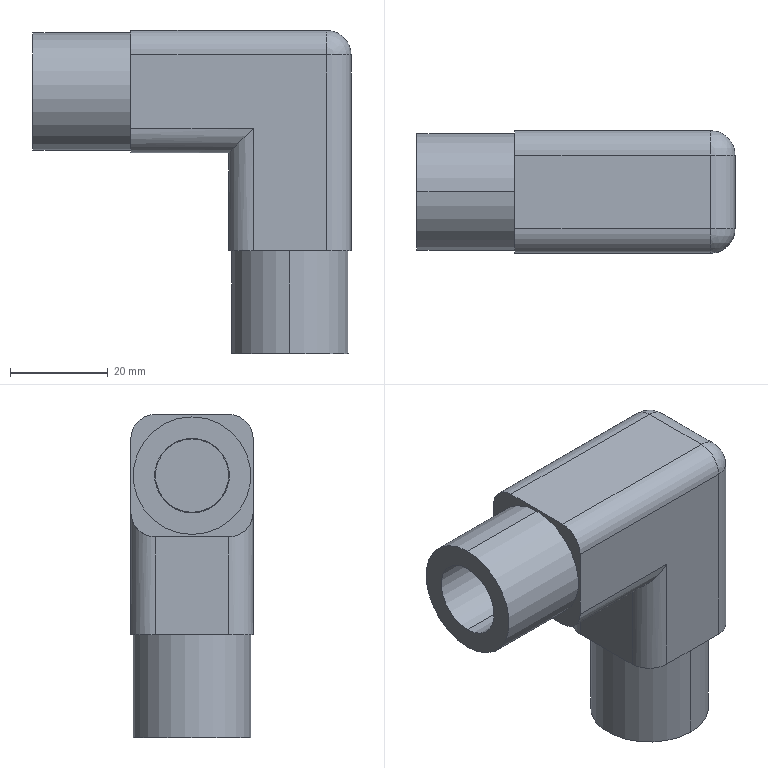Part | STEP file | GLSJ-10-35 | 1 solid | 40 faces | box 65 x 25 x 66 mm | volume 38293 mm3 | cylinder 21 | plane 13 | cone 4 | sphere 2 | commonest cylinder face diameters 10 x9 15 x4 15.25 x4 24 x4